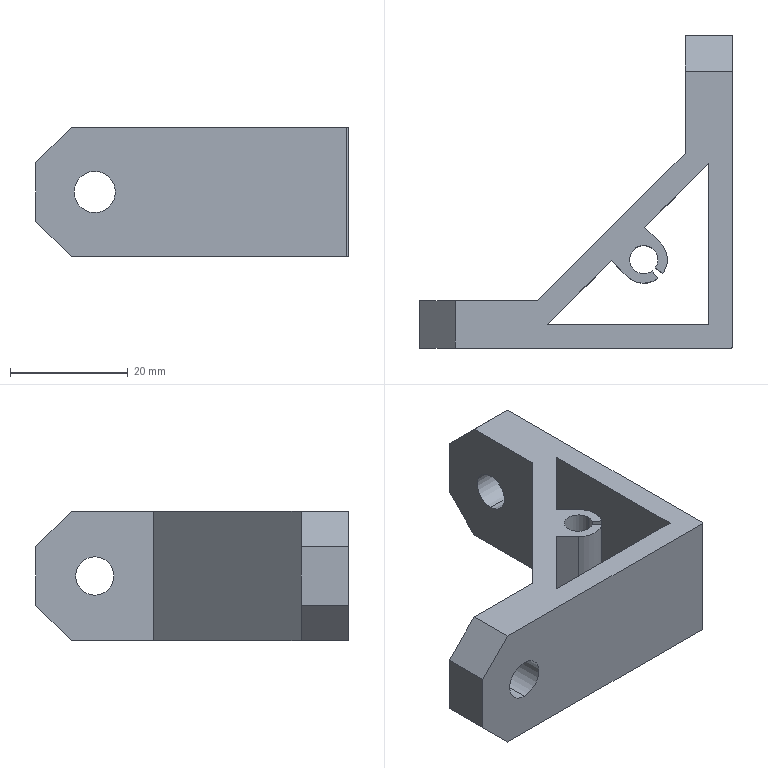Part | SolidWorks | features ICE 3, Chamfer 1, Extrusion 1 | 1 solid | 80 faces | box 53 x 53 x 22 mm | volume 15531 mm3 | plane 54 | spline 16 | cylinder 10 | commonest cylinder face diameters 4.8 x3 6.5 x2 7 x2 8 x2 0.474 x1